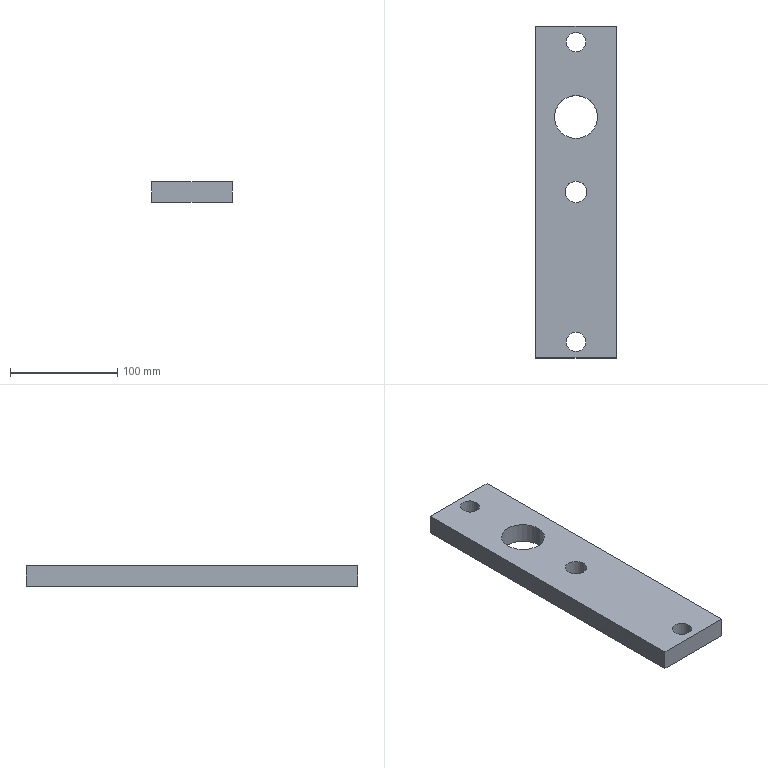Part | NX | features solid 2 | 1 solid | 10 faces | box 75 x 310 x 19 mm | volume 402235 mm3 | plane 6 | cylinder 4 | commonest cylinder face diameters 18 x2 20 x1 40 x1
STEP:
#1=CARTESIAN_POINT('',(255.,80.,-90.));
#2=VERTEX_POINT('',#1);
#3=CARTESIAN_POINT('',(255.,60.,-90.));
#4=DIRECTION('',(0.,0.,-1.));
#5=DIRECTION('',(0.,1.,0.));
#6=AXIS2_PLACEMENT_3D('',#3,#4,#5);
#7=CIRCLE('',#6,20.);
#8=EDGE_CURVE('',#2,#2,#7,.T.);
#9=ORIENTED_EDGE('',*,*,#8,.F.);
#10=EDGE_LOOP('',(#9));
#11=FACE_BOUND('',#10,.T.);
#12=CARTESIAN_POINT('',(255.,0.,-90.));
#13=VERTEX_POINT('',#12);
#14=CARTESIAN_POINT('',(255.,-10.,-90.));
#15=DIRECTION('',(0.,0.,1.));
#16=DIRECTION('',(0.,1.,0.));
#17=AXIS2_PLACEMENT_3D('',#14,#15,#16);
#18=CIRCLE('',#17,10.);
#19=EDGE_CURVE('',#13,#13,#18,.T.);
#20=ORIENTED_EDGE('',*,*,#19,.T.);
#21=EDGE_LOOP('',(#20));
#22=FACE_BOUND('',#21,.T.);
#23=CARTESIAN_POINT('',(217.5,145.,-90.));
#24=VERTEX_POINT('',#23);
#25=CARTESIAN_POINT('',(292.5,145.,-90.));
#26=VERTEX_POINT('',#25);
#27=CARTESIAN_POINT('',(217.5,145.,-90.));
#28=DIRECTION('',(1.,0.,0.));
#29=VECTOR('',#28,1000.);
#30=LINE('',#27,#29);
#31=EDGE_CURVE('',#24,#26,#30,.T.);
#32=ORIENTED_EDGE('',*,*,#31,.T.);
#33=CARTESIAN_POINT('',(292.5,-165.,-90.));
#34=VERTEX_POINT('',#33);
#35=CARTESIAN_POINT('',(292.5,145.,-90.));
#36=DIRECTION('',(0.,-1.,0.));
#37=VECTOR('',#36,1000.);
#38=LINE('',#35,#37);
#39=EDGE_CURVE('',#26,#34,#38,.T.);
#40=ORIENTED_EDGE('',*,*,#39,.T.);
#41=CARTESIAN_POINT('',(217.5,-165.,-90.));
#42=VERTEX_POINT('',#41);
#43=CARTESIAN_POINT('',(292.5,-165.,-90.));
#44=DIRECTION('',(-1.,0.,0.));
#45=VECTOR('',#44,1000.);
#46=LINE('',#43,#45);
#47=EDGE_CURVE('',#34,#42,#46,.T.);
#48=ORIENTED_EDGE('',*,*,#47,.T.);
#49=CARTESIAN_POINT('',(217.5,-165.,-90.));
#50=DIRECTION('',(0.,1.,0.));
#51=VECTOR('',#50,1000.);
#52=LINE('',#49,#51);
#53=EDGE_CURVE('',#42,#24,#52,.T.);
#54=ORIENTED_EDGE('',*,*,#53,.T.);
#55=EDGE_LOOP('',(#32,#40,#48,#54));
#56=FACE_BOUND('',#55,.T.);
#57=CARTESIAN_POINT('',(255.,-141.,-90.));
#58=VERTEX_POINT('',#57);
#59=CARTESIAN_POINT('',(255.,-150.,-90.));
#60=DIRECTION('',(0.,0.,1.));
#61=DIRECTION('',(0.,1.,0.));
#62=AXIS2_PLACEMENT_3D('',#59,#60,#61);
#63=CIRCLE('',#62,9.);
#64=EDGE_CURVE('',#58,#58,#63,.T.);
#65=ORIENTED_EDGE('',*,*,#64,.T.);
#66=EDGE_LOOP('',(#65));
#67=FACE_BOUND('',#66,.T.);
#68=CARTESIAN_POINT('',(255.,139.,-90.));
#69=VERTEX_POINT('',#68);
#70=CARTESIAN_POINT('',(255.,130.,-90.));
#71=DIRECTION('',(0.,0.,1.));
#72=DIRECTION('',(0.,1.,0.));
#73=AXIS2_PLACEMENT_3D('',#70,#71,#72);
#74=CIRCLE('',#73,9.);
#75=EDGE_CURVE('',#69,#69,#74,.F.);
#76=ORIENTED_EDGE('',*,*,#75,.F.);
#77=EDGE_LOOP('',(#76));
#78=FACE_BOUND('',#77,.T.);
#79=CARTESIAN_POINT('',(217.5,145.,-90.));
#80=DIRECTION('',(0.,0.,1.));
#81=DIRECTION('',(0.,1.,0.));
#82=AXIS2_PLACEMENT_3D('',#79,#80,#81);
#83=PLANE('',#82);
#84=ADVANCED_FACE('',(#11,#22,#56,#67,#78),#83,.F.);
#85=CARTESIAN_POINT('',(255.,80.,-71.));
#86=VERTEX_POINT('',#85);
#87=CARTESIAN_POINT('',(255.,60.,-71.));
#88=DIRECTION('',(0.,0.,-1.));
#89=DIRECTION('',(0.,1.,0.));
#90=AXIS2_PLACEMENT_3D('',#87,#88,#89);
#91=CIRCLE('',#90,20.);
#92=EDGE_CURVE('',#86,#86,#91,.T.);
#93=ORIENTED_EDGE('',*,*,#92,.T.);
#94=EDGE_LOOP('',(#93));
#95=FACE_BOUND('',#94,.T.);
#96=CARTESIAN_POINT('',(255.,0.,-71.));
#97=VERTEX_POINT('',#96);
#98=CARTESIAN_POINT('',(255.,-10.,-71.));
#99=DIRECTION('',(0.,0.,1.));
#100=DIRECTION('',(0.,1.,0.));
#101=AXIS2_PLACEMENT_3D('',#98,#99,#100);
#102=CIRCLE('',#101,10.);
#103=EDGE_CURVE('',#97,#97,#102,.F.);
#104=ORIENTED_EDGE('',*,*,#103,.T.);
#105=EDGE_LOOP('',(#104));
#106=FACE_BOUND('',#105,.T.);
#107=CARTESIAN_POINT('',(217.5,145.,-71.));
#108=VERTEX_POINT('',#107);
#109=CARTESIAN_POINT('',(292.5,145.,-71.));
#110=VERTEX_POINT('',#109);
#111=CARTESIAN_POINT('',(217.5,145.,-71.));
#112=DIRECTION('',(1.,0.,0.));
#113=VECTOR('',#112,1000.);
#114=LINE('',#111,#113);
#115=EDGE_CURVE('',#108,#110,#114,.T.);
#116=ORIENTED_EDGE('',*,*,#115,.F.);
#117=CARTESIAN_POINT('',(217.5,-165.,-71.));
#118=VERTEX_POINT('',#117);
#119=CARTESIAN_POINT('',(217.5,-165.,-71.));
#120=DIRECTION('',(0.,1.,0.));
#121=VECTOR('',#120,1000.);
#122=LINE('',#119,#121);
#123=EDGE_CURVE('',#118,#108,#122,.T.);
#124=ORIENTED_EDGE('',*,*,#123,.F.);
#125=CARTESIAN_POINT('',(292.5,-165.,-71.));
#126=VERTEX_POINT('',#125);
#127=CARTESIAN_POINT('',(292.5,-165.,-71.));
#128=DIRECTION('',(-1.,0.,0.));
#129=VECTOR('',#128,1000.);
#130=LINE('',#127,#129);
#131=EDGE_CURVE('',#126,#118,#130,.T.);
#132=ORIENTED_EDGE('',*,*,#131,.F.);
#133=CARTESIAN_POINT('',(292.5,145.,-71.));
#134=DIRECTION('',(0.,-1.,0.));
#135=VECTOR('',#134,1000.);
#136=LINE('',#133,#135);
#137=EDGE_CURVE('',#110,#126,#136,.T.);
#138=ORIENTED_EDGE('',*,*,#137,.F.);
#139=EDGE_LOOP('',(#116,#124,#132,#138));
#140=FACE_BOUND('',#139,.T.);
#141=CARTESIAN_POINT('',(255.,-141.,-71.));
#142=VERTEX_POINT('',#141);
#143=CARTESIAN_POINT('',(255.,-150.,-71.));
#144=DIRECTION('',(0.,0.,1.));
#145=DIRECTION('',(0.,1.,0.));
#146=AXIS2_PLACEMENT_3D('',#143,#144,#145);
#147=CIRCLE('',#146,9.);
#148=EDGE_CURVE('',#142,#142,#147,.T.);
#149=ORIENTED_EDGE('',*,*,#148,.F.);
#150=EDGE_LOOP('',(#149));
#151=FACE_BOUND('',#150,.T.);
#152=CARTESIAN_POINT('',(255.,139.,-71.));
#153=VERTEX_POINT('',#152);
#154=CARTESIAN_POINT('',(255.,130.,-71.));
#155=DIRECTION('',(0.,0.,1.));
#156=DIRECTION('',(0.,1.,0.));
#157=AXIS2_PLACEMENT_3D('',#154,#155,#156);
#158=CIRCLE('',#157,9.);
#159=EDGE_CURVE('',#153,#153,#158,.F.);
#160=ORIENTED_EDGE('',*,*,#159,.T.);
#161=EDGE_LOOP('',(#160));
#162=FACE_BOUND('',#161,.T.);
#163=CARTESIAN_POINT('',(217.5,145.,-71.));
#164=DIRECTION('',(0.,0.,1.));
#165=DIRECTION('',(0.,1.,0.));
#166=AXIS2_PLACEMENT_3D('',#163,#164,#165);
#167=PLANE('',#166);
#168=ADVANCED_FACE('',(#95,#106,#140,#151,#162),#167,.T.);
#169=ORIENTED_EDGE('',*,*,#115,.T.);
#170=CARTESIAN_POINT('',(292.5,145.,-90.));
#171=DIRECTION('',(0.,0.,1.));
#172=VECTOR('',#171,1000.);
#173=LINE('',#170,#172);
#174=EDGE_CURVE('',#26,#110,#173,.T.);
#175=ORIENTED_EDGE('',*,*,#174,.F.);
#176=ORIENTED_EDGE('',*,*,#31,.F.);
#177=CARTESIAN_POINT('',(217.5,145.,-90.));
#178=DIRECTION('',(0.,0.,1.));
#179=VECTOR('',#178,1000.);
#180=LINE('',#177,#179);
#181=EDGE_CURVE('',#24,#108,#180,.T.);
#182=ORIENTED_EDGE('',*,*,#181,.T.);
#183=EDGE_LOOP('',(#169,#175,#176,#182));
#184=FACE_BOUND('',#183,.T.);
#185=CARTESIAN_POINT('',(217.5,145.,-90.));
#186=DIRECTION('',(0.,-1.,0.));
#187=DIRECTION('',(0.,0.,1.));
#188=AXIS2_PLACEMENT_3D('',#185,#186,#187);
#189=PLANE('',#188);
#190=ADVANCED_FACE('',(#184),#189,.F.);
#191=ORIENTED_EDGE('',*,*,#137,.T.);
#192=CARTESIAN_POINT('',(292.5,-165.,-90.));
#193=DIRECTION('',(0.,0.,1.));
#194=VECTOR('',#193,1000.);
#195=LINE('',#192,#194);
#196=EDGE_CURVE('',#34,#126,#195,.T.);
#197=ORIENTED_EDGE('',*,*,#196,.F.);
#198=ORIENTED_EDGE('',*,*,#39,.F.);
#199=ORIENTED_EDGE('',*,*,#174,.T.);
#200=EDGE_LOOP('',(#191,#197,#198,#199));
#201=FACE_BOUND('',#200,.T.);
#202=CARTESIAN_POINT('',(292.5,145.,-90.));
#203=DIRECTION('',(-1.,0.,0.));
#204=DIRECTION('',(0.,-1.,0.));
#205=AXIS2_PLACEMENT_3D('',#202,#203,#204);
#206=PLANE('',#205);
#207=ADVANCED_FACE('',(#201),#206,.F.);
#208=ORIENTED_EDGE('',*,*,#131,.T.);
#209=CARTESIAN_POINT('',(217.5,-165.,-90.));
#210=DIRECTION('',(0.,0.,1.));
#211=VECTOR('',#210,1000.);
#212=LINE('',#209,#211);
#213=EDGE_CURVE('',#42,#118,#212,.T.);
#214=ORIENTED_EDGE('',*,*,#213,.F.);
#215=ORIENTED_EDGE('',*,*,#47,.F.);
#216=ORIENTED_EDGE('',*,*,#196,.T.);
#217=EDGE_LOOP('',(#208,#214,#215,#216));
#218=FACE_BOUND('',#217,.T.);
#219=CARTESIAN_POINT('',(292.5,-165.,-90.));
#220=DIRECTION('',(0.,1.,0.));
#221=DIRECTION('',(0.,0.,-1.));
#222=AXIS2_PLACEMENT_3D('',#219,#220,#221);
#223=PLANE('',#222);
#224=ADVANCED_FACE('',(#218),#223,.F.);
#225=ORIENTED_EDGE('',*,*,#123,.T.);
#226=ORIENTED_EDGE('',*,*,#181,.F.);
#227=ORIENTED_EDGE('',*,*,#53,.F.);
#228=ORIENTED_EDGE('',*,*,#213,.T.);
#229=EDGE_LOOP('',(#225,#226,#227,#228));
#230=FACE_BOUND('',#229,.T.);
#231=CARTESIAN_POINT('',(217.5,-165.,-90.));
#232=DIRECTION('',(1.,0.,0.));
#233=DIRECTION('',(0.,0.,-1.));
#234=AXIS2_PLACEMENT_3D('',#231,#232,#233);
#235=PLANE('',#234);
#236=ADVANCED_FACE('',(#230),#235,.F.);
#237=ORIENTED_EDGE('',*,*,#19,.F.);
#238=EDGE_LOOP('',(#237));
#239=FACE_BOUND('',#238,.T.);
#240=ORIENTED_EDGE('',*,*,#103,.F.);
#241=EDGE_LOOP('',(#240));
#242=FACE_BOUND('',#241,.T.);
#243=CARTESIAN_POINT('',(255.,-10.,-71.));
#244=DIRECTION('',(0.,0.,-1.));
#245=DIRECTION('',(0.,1.,0.));
#246=AXIS2_PLACEMENT_3D('',#243,#244,#245);
#247=CYLINDRICAL_SURFACE('',#246,10.);
#248=ADVANCED_FACE('',(#239,#242),#247,.F.);
#249=ORIENTED_EDGE('',*,*,#8,.T.);
#250=EDGE_LOOP('',(#249));
#251=FACE_BOUND('',#250,.T.);
#252=ORIENTED_EDGE('',*,*,#92,.F.);
#253=EDGE_LOOP('',(#252));
#254=FACE_BOUND('',#253,.T.);
#255=CARTESIAN_POINT('',(255.,60.,-90.));
#256=DIRECTION('',(0.,0.,1.));
#257=DIRECTION('',(0.,1.,0.));
#258=AXIS2_PLACEMENT_3D('',#255,#256,#257);
#259=CYLINDRICAL_SURFACE('',#258,20.);
#260=ADVANCED_FACE('',(#251,#254),#259,.F.);
#261=ORIENTED_EDGE('',*,*,#148,.T.);
#262=EDGE_LOOP('',(#261));
#263=FACE_BOUND('',#262,.T.);
#264=ORIENTED_EDGE('',*,*,#64,.F.);
#265=EDGE_LOOP('',(#264));
#266=FACE_BOUND('',#265,.T.);
#267=CARTESIAN_POINT('',(255.,-150.,-220.));
#268=DIRECTION('',(0.,0.,1.));
#269=DIRECTION('',(0.,1.,0.));
#270=AXIS2_PLACEMENT_3D('',#267,#268,#269);
#271=CYLINDRICAL_SURFACE('',#270,9.);
#272=ADVANCED_FACE('',(#263,#266),#271,.F.);
#273=ORIENTED_EDGE('',*,*,#159,.F.);
#274=EDGE_LOOP('',(#273));
#275=FACE_BOUND('',#274,.T.);
#276=ORIENTED_EDGE('',*,*,#75,.T.);
#277=EDGE_LOOP('',(#276));
#278=FACE_BOUND('',#277,.T.);
#279=CARTESIAN_POINT('',(255.,130.,-220.));
#280=DIRECTION('',(0.,0.,1.));
#281=DIRECTION('',(0.,1.,0.));
#282=AXIS2_PLACEMENT_3D('',#279,#280,#281);
#283=CYLINDRICAL_SURFACE('',#282,9.);
#284=ADVANCED_FACE('',(#275,#278),#283,.F.);
#285=CLOSED_SHELL('',(#84,#168,#190,#207,#224,#236,#248,#260,#272,#284));
#286=MANIFOLD_SOLID_BREP('',#285);
#287=(LENGTH_UNIT()NAMED_UNIT(*)SI_UNIT(.MILLI.,.METRE.));
#288=UNCERTAINTY_MEASURE_WITH_UNIT(LENGTH_MEASURE(0.00001),#287,'','');
#289=(NAMED_UNIT(*)PLANE_ANGLE_UNIT()SI_UNIT($,.RADIAN.));
#290=(NAMED_UNIT(*)SI_UNIT($,.STERADIAN.)SOLID_ANGLE_UNIT());
#291=(GEOMETRIC_REPRESENTATION_CONTEXT(3)GLOBAL_UNCERTAINTY_ASSIGNED_CONTEXT((#288))GLOBAL_UNIT_ASSIGNED_CONTEXT((#287,#289,#290))REPRESENTATION_CONTEXT('',''));
#292=ADVANCED_BREP_SHAPE_REPRESENTATION('',(#286),#291);